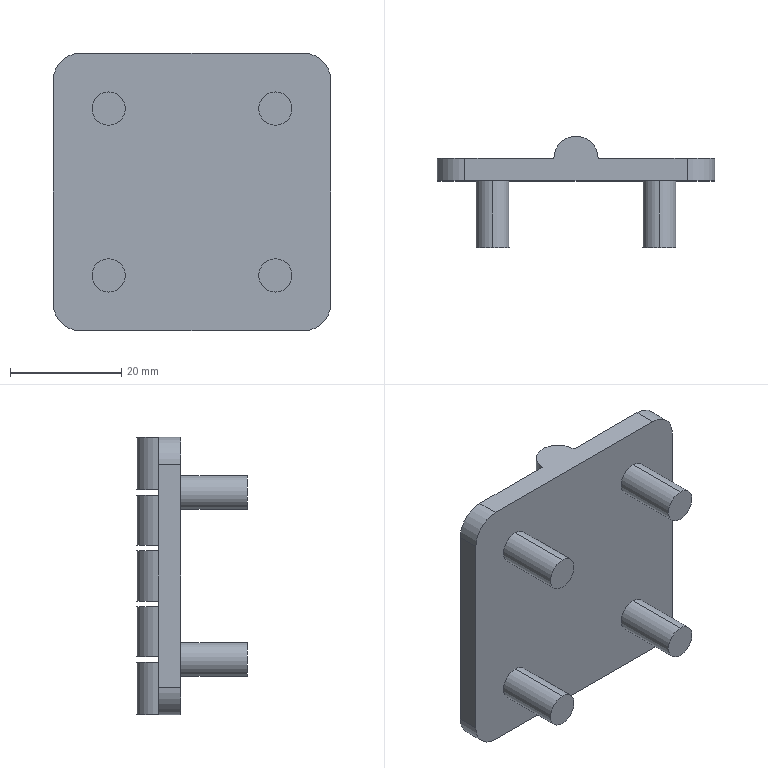Part | NX | features solid 2 | 1 solid | 35 faces | box 50 x 20 x 50 mm | volume 12427 mm3 | plane 18 | cylinder 17 | commonest cylinder face diameters 6 x8 8 x5 10 x4
STEP:
#1=CARTESIAN_POINT('',(675.,534.,662.));
#2=VERTEX_POINT('',#1);
#3=CARTESIAN_POINT('',(667.,534.,662.));
#4=VERTEX_POINT('',#3);
#5=CARTESIAN_POINT('',(671.,534.,662.));
#6=DIRECTION('',(0.,0.,1.));
#7=DIRECTION('',(0.,1.,0.));
#8=AXIS2_PLACEMENT_3D('',#5,#6,#7);
#9=CIRCLE('',#8,4.);
#10=EDGE_CURVE('',#2,#4,#9,.T.);
#11=ORIENTED_EDGE('',*,*,#10,.T.);
#12=CARTESIAN_POINT('',(676.528,534.,662.));
#13=DIRECTION('',(-1.,0.,0.));
#14=VECTOR('',#13,1000.);
#15=LINE('',#12,#14);
#16=EDGE_CURVE('',#2,#4,#15,.T.);
#17=ORIENTED_EDGE('',*,*,#16,.F.);
#18=EDGE_LOOP('',(#11,#17));
#19=FACE_BOUND('',#18,.T.);
#20=CARTESIAN_POINT('',(676.528,607.485,662.));
#21=DIRECTION('',(0.,0.,1.));
#22=DIRECTION('',(1.,0.,0.));
#23=AXIS2_PLACEMENT_3D('',#20,#21,#22);
#24=PLANE('',#23);
#25=ADVANCED_FACE('',(#19),#24,.T.);
#26=CARTESIAN_POINT('',(667.,534.,663.));
#27=VERTEX_POINT('',#26);
#28=CARTESIAN_POINT('',(675.,534.,663.));
#29=VERTEX_POINT('',#28);
#30=CARTESIAN_POINT('',(671.,534.,663.));
#31=DIRECTION('',(0.,0.,-1.));
#32=DIRECTION('',(0.,-1.,0.));
#33=AXIS2_PLACEMENT_3D('',#30,#31,#32);
#34=CIRCLE('',#33,4.);
#35=EDGE_CURVE('',#27,#29,#34,.T.);
#36=ORIENTED_EDGE('',*,*,#35,.T.);
#37=CARTESIAN_POINT('',(676.528,534.,663.));
#38=DIRECTION('',(1.,0.,0.));
#39=VECTOR('',#38,1000.);
#40=LINE('',#37,#39);
#41=EDGE_CURVE('',#27,#29,#40,.T.);
#42=ORIENTED_EDGE('',*,*,#41,.F.);
#43=EDGE_LOOP('',(#36,#42));
#44=FACE_BOUND('',#43,.T.);
#45=CARTESIAN_POINT('',(676.528,607.485,663.));
#46=DIRECTION('',(0.,0.,-1.));
#47=DIRECTION('',(0.,-1.,0.));
#48=AXIS2_PLACEMENT_3D('',#45,#46,#47);
#49=PLANE('',#48);
#50=ADVANCED_FACE('',(#44),#49,.T.);
#51=CARTESIAN_POINT('',(675.,534.,632.));
#52=VERTEX_POINT('',#51);
#53=CARTESIAN_POINT('',(667.,534.,632.));
#54=VERTEX_POINT('',#53);
#55=CARTESIAN_POINT('',(671.,534.,632.));
#56=DIRECTION('',(0.,0.,1.));
#57=DIRECTION('',(0.,1.,0.));
#58=AXIS2_PLACEMENT_3D('',#55,#56,#57);
#59=CIRCLE('',#58,4.);
#60=EDGE_CURVE('',#52,#54,#59,.T.);
#61=ORIENTED_EDGE('',*,*,#60,.T.);
#62=CARTESIAN_POINT('',(676.528,534.,632.));
#63=DIRECTION('',(-1.,0.,0.));
#64=VECTOR('',#63,1000.);
#65=LINE('',#62,#64);
#66=EDGE_CURVE('',#52,#54,#65,.T.);
#67=ORIENTED_EDGE('',*,*,#66,.F.);
#68=EDGE_LOOP('',(#61,#67));
#69=FACE_BOUND('',#68,.T.);
#70=CARTESIAN_POINT('',(676.528,607.485,632.));
#71=DIRECTION('',(0.,0.,1.));
#72=DIRECTION('',(1.,0.,0.));
#73=AXIS2_PLACEMENT_3D('',#70,#71,#72);
#74=PLANE('',#73);
#75=ADVANCED_FACE('',(#69),#74,.T.);
#76=CARTESIAN_POINT('',(667.,534.,633.));
#77=VERTEX_POINT('',#76);
#78=CARTESIAN_POINT('',(675.,534.,633.));
#79=VERTEX_POINT('',#78);
#80=CARTESIAN_POINT('',(671.,534.,633.));
#81=DIRECTION('',(0.,0.,-1.));
#82=DIRECTION('',(0.,-1.,0.));
#83=AXIS2_PLACEMENT_3D('',#80,#81,#82);
#84=CIRCLE('',#83,4.);
#85=EDGE_CURVE('',#77,#79,#84,.T.);
#86=ORIENTED_EDGE('',*,*,#85,.T.);
#87=CARTESIAN_POINT('',(676.528,534.,633.));
#88=DIRECTION('',(1.,0.,0.));
#89=VECTOR('',#88,1000.);
#90=LINE('',#87,#89);
#91=EDGE_CURVE('',#77,#79,#90,.T.);
#92=ORIENTED_EDGE('',*,*,#91,.F.);
#93=EDGE_LOOP('',(#86,#92));
#94=FACE_BOUND('',#93,.T.);
#95=CARTESIAN_POINT('',(676.528,607.485,633.));
#96=DIRECTION('',(0.,0.,-1.));
#97=DIRECTION('',(0.,-1.,0.));
#98=AXIS2_PLACEMENT_3D('',#95,#96,#97);
#99=PLANE('',#98);
#100=ADVANCED_FACE('',(#94),#99,.T.);
#101=CARTESIAN_POINT('',(675.,534.,642.));
#102=VERTEX_POINT('',#101);
#103=CARTESIAN_POINT('',(667.,534.,642.));
#104=VERTEX_POINT('',#103);
#105=CARTESIAN_POINT('',(671.,534.,642.));
#106=DIRECTION('',(0.,0.,1.));
#107=DIRECTION('',(0.,1.,0.));
#108=AXIS2_PLACEMENT_3D('',#105,#106,#107);
#109=CIRCLE('',#108,4.);
#110=EDGE_CURVE('',#102,#104,#109,.T.);
#111=ORIENTED_EDGE('',*,*,#110,.T.);
#112=CARTESIAN_POINT('',(676.528,534.,642.));
#113=DIRECTION('',(-1.,0.,0.));
#114=VECTOR('',#113,1000.);
#115=LINE('',#112,#114);
#116=EDGE_CURVE('',#102,#104,#115,.T.);
#117=ORIENTED_EDGE('',*,*,#116,.F.);
#118=EDGE_LOOP('',(#111,#117));
#119=FACE_BOUND('',#118,.T.);
#120=CARTESIAN_POINT('',(676.528,607.485,642.));
#121=DIRECTION('',(0.,0.,1.));
#122=DIRECTION('',(1.,0.,0.));
#123=AXIS2_PLACEMENT_3D('',#120,#121,#122);
#124=PLANE('',#123);
#125=ADVANCED_FACE('',(#119),#124,.T.);
#126=CARTESIAN_POINT('',(667.,534.,643.));
#127=VERTEX_POINT('',#126);
#128=CARTESIAN_POINT('',(675.,534.,643.));
#129=VERTEX_POINT('',#128);
#130=CARTESIAN_POINT('',(671.,534.,643.));
#131=DIRECTION('',(0.,0.,-1.));
#132=DIRECTION('',(0.,-1.,0.));
#133=AXIS2_PLACEMENT_3D('',#130,#131,#132);
#134=CIRCLE('',#133,4.);
#135=EDGE_CURVE('',#127,#129,#134,.T.);
#136=ORIENTED_EDGE('',*,*,#135,.T.);
#137=CARTESIAN_POINT('',(676.528,534.,643.));
#138=DIRECTION('',(1.,0.,0.));
#139=VECTOR('',#138,1000.);
#140=LINE('',#137,#139);
#141=EDGE_CURVE('',#127,#129,#140,.T.);
#142=ORIENTED_EDGE('',*,*,#141,.F.);
#143=EDGE_LOOP('',(#136,#142));
#144=FACE_BOUND('',#143,.T.);
#145=CARTESIAN_POINT('',(676.528,607.485,643.));
#146=DIRECTION('',(0.,0.,-1.));
#147=DIRECTION('',(0.,-1.,0.));
#148=AXIS2_PLACEMENT_3D('',#145,#146,#147);
#149=PLANE('',#148);
#150=ADVANCED_FACE('',(#144),#149,.T.);
#151=CARTESIAN_POINT('',(675.,534.,652.));
#152=VERTEX_POINT('',#151);
#153=CARTESIAN_POINT('',(667.,534.,652.));
#154=VERTEX_POINT('',#153);
#155=CARTESIAN_POINT('',(671.,534.,652.));
#156=DIRECTION('',(0.,0.,1.));
#157=DIRECTION('',(0.,1.,0.));
#158=AXIS2_PLACEMENT_3D('',#155,#156,#157);
#159=CIRCLE('',#158,4.);
#160=EDGE_CURVE('',#152,#154,#159,.T.);
#161=ORIENTED_EDGE('',*,*,#160,.T.);
#162=CARTESIAN_POINT('',(676.528,534.,652.));
#163=DIRECTION('',(-1.,0.,0.));
#164=VECTOR('',#163,1000.);
#165=LINE('',#162,#164);
#166=EDGE_CURVE('',#152,#154,#165,.T.);
#167=ORIENTED_EDGE('',*,*,#166,.F.);
#168=EDGE_LOOP('',(#161,#167));
#169=FACE_BOUND('',#168,.T.);
#170=CARTESIAN_POINT('',(676.528,607.485,652.));
#171=DIRECTION('',(0.,0.,1.));
#172=DIRECTION('',(1.,0.,0.));
#173=AXIS2_PLACEMENT_3D('',#170,#171,#172);
#174=PLANE('',#173);
#175=ADVANCED_FACE('',(#169),#174,.T.);
#176=CARTESIAN_POINT('',(667.,534.,653.));
#177=VERTEX_POINT('',#176);
#178=CARTESIAN_POINT('',(675.,534.,653.));
#179=VERTEX_POINT('',#178);
#180=CARTESIAN_POINT('',(671.,534.,653.));
#181=DIRECTION('',(0.,0.,-1.));
#182=DIRECTION('',(0.,-1.,0.));
#183=AXIS2_PLACEMENT_3D('',#180,#181,#182);
#184=CIRCLE('',#183,4.);
#185=EDGE_CURVE('',#177,#179,#184,.T.);
#186=ORIENTED_EDGE('',*,*,#185,.T.);
#187=CARTESIAN_POINT('',(676.528,534.,653.));
#188=DIRECTION('',(1.,0.,0.));
#189=VECTOR('',#188,1000.);
#190=LINE('',#187,#189);
#191=EDGE_CURVE('',#177,#179,#190,.T.);
#192=ORIENTED_EDGE('',*,*,#191,.F.);
#193=EDGE_LOOP('',(#186,#192));
#194=FACE_BOUND('',#193,.T.);
#195=CARTESIAN_POINT('',(676.528,607.485,653.));
#196=DIRECTION('',(0.,0.,-1.));
#197=DIRECTION('',(0.,-1.,0.));
#198=AXIS2_PLACEMENT_3D('',#195,#196,#197);
#199=PLANE('',#198);
#200=ADVANCED_FACE('',(#194),#199,.T.);
#201=CARTESIAN_POINT('',(686.,518.,629.5));
#202=VERTEX_POINT('',#201);
#203=CARTESIAN_POINT('',(686.,518.,635.5));
#204=VERTEX_POINT('',#203);
#205=CARTESIAN_POINT('',(686.,518.,632.5));
#206=DIRECTION('',(0.,1.,0.));
#207=DIRECTION('',(-1.,0.,0.));
#208=AXIS2_PLACEMENT_3D('',#205,#206,#207);
#209=CIRCLE('',#208,3.);
#210=EDGE_CURVE('',#202,#204,#209,.T.);
#211=ORIENTED_EDGE('',*,*,#210,.F.);
#212=CARTESIAN_POINT('',(686.,518.,632.5));
#213=DIRECTION('',(0.,1.,0.));
#214=DIRECTION('',(-1.,0.,0.));
#215=AXIS2_PLACEMENT_3D('',#212,#213,#214);
#216=CIRCLE('',#215,3.);
#217=EDGE_CURVE('',#204,#202,#216,.T.);
#218=ORIENTED_EDGE('',*,*,#217,.F.);
#219=EDGE_LOOP('',(#211,#218));
#220=FACE_BOUND('',#219,.T.);
#221=CARTESIAN_POINT('',(686.,518.,632.5));
#222=DIRECTION('',(0.,1.,0.));
#223=DIRECTION('',(1.,0.,0.));
#224=AXIS2_PLACEMENT_3D('',#221,#222,#223);
#225=PLANE('',#224);
#226=ADVANCED_FACE('',(#220),#225,.F.);
#227=CARTESIAN_POINT('',(686.,530.,635.5));
#228=VERTEX_POINT('',#227);
#229=CARTESIAN_POINT('',(686.,518.,635.5));
#230=DIRECTION('',(0.,1.,0.));
#231=VECTOR('',#230,1000.);
#232=LINE('',#229,#231);
#233=EDGE_CURVE('',#228,#204,#232,.F.);
#234=ORIENTED_EDGE('',*,*,#233,.T.);
#235=ORIENTED_EDGE('',*,*,#217,.T.);
#236=CARTESIAN_POINT('',(686.,530.,629.5));
#237=VERTEX_POINT('',#236);
#238=CARTESIAN_POINT('',(686.,518.,629.5));
#239=DIRECTION('',(0.,1.,0.));
#240=VECTOR('',#239,1000.);
#241=LINE('',#238,#240);
#242=EDGE_CURVE('',#202,#237,#241,.T.);
#243=ORIENTED_EDGE('',*,*,#242,.T.);
#244=CARTESIAN_POINT('',(686.,530.,632.5));
#245=DIRECTION('',(0.,-1.,0.));
#246=DIRECTION('',(0.,0.,1.));
#247=AXIS2_PLACEMENT_3D('',#244,#245,#246);
#248=CIRCLE('',#247,3.);
#249=EDGE_CURVE('',#237,#228,#248,.T.);
#250=ORIENTED_EDGE('',*,*,#249,.T.);
#251=EDGE_LOOP('',(#234,#235,#243,#250));
#252=FACE_BOUND('',#251,.T.);
#253=CARTESIAN_POINT('',(686.,518.,632.5));
#254=DIRECTION('',(0.,1.,0.));
#255=DIRECTION('',(0.,0.,-1.));
#256=AXIS2_PLACEMENT_3D('',#253,#254,#255);
#257=CYLINDRICAL_SURFACE('',#256,3.);
#258=ADVANCED_FACE('',(#252),#257,.T.);
#259=CARTESIAN_POINT('',(686.,518.,659.5));
#260=VERTEX_POINT('',#259);
#261=CARTESIAN_POINT('',(686.,518.,665.5));
#262=VERTEX_POINT('',#261);
#263=CARTESIAN_POINT('',(686.,518.,662.5));
#264=DIRECTION('',(0.,1.,0.));
#265=DIRECTION('',(-1.,0.,0.));
#266=AXIS2_PLACEMENT_3D('',#263,#264,#265);
#267=CIRCLE('',#266,3.);
#268=EDGE_CURVE('',#260,#262,#267,.T.);
#269=ORIENTED_EDGE('',*,*,#268,.F.);
#270=CARTESIAN_POINT('',(686.,518.,662.5));
#271=DIRECTION('',(0.,1.,0.));
#272=DIRECTION('',(-1.,0.,0.));
#273=AXIS2_PLACEMENT_3D('',#270,#271,#272);
#274=CIRCLE('',#273,3.);
#275=EDGE_CURVE('',#262,#260,#274,.T.);
#276=ORIENTED_EDGE('',*,*,#275,.F.);
#277=EDGE_LOOP('',(#269,#276));
#278=FACE_BOUND('',#277,.T.);
#279=CARTESIAN_POINT('',(686.,518.,662.5));
#280=DIRECTION('',(0.,1.,0.));
#281=DIRECTION('',(1.,0.,0.));
#282=AXIS2_PLACEMENT_3D('',#279,#280,#281);
#283=PLANE('',#282);
#284=ADVANCED_FACE('',(#278),#283,.F.);
#285=CARTESIAN_POINT('',(686.,530.,665.5));
#286=VERTEX_POINT('',#285);
#287=CARTESIAN_POINT('',(686.,518.,665.5));
#288=DIRECTION('',(0.,1.,0.));
#289=VECTOR('',#288,1000.);
#290=LINE('',#287,#289);
#291=EDGE_CURVE('',#286,#262,#290,.F.);
#292=ORIENTED_EDGE('',*,*,#291,.T.);
#293=ORIENTED_EDGE('',*,*,#275,.T.);
#294=CARTESIAN_POINT('',(686.,530.,659.5));
#295=VERTEX_POINT('',#294);
#296=CARTESIAN_POINT('',(686.,518.,659.5));
#297=DIRECTION('',(0.,1.,0.));
#298=VECTOR('',#297,1000.);
#299=LINE('',#296,#298);
#300=EDGE_CURVE('',#260,#295,#299,.T.);
#301=ORIENTED_EDGE('',*,*,#300,.T.);
#302=CARTESIAN_POINT('',(686.,530.,662.5));
#303=DIRECTION('',(0.,-1.,0.));
#304=DIRECTION('',(0.,0.,1.));
#305=AXIS2_PLACEMENT_3D('',#302,#303,#304);
#306=CIRCLE('',#305,3.);
#307=EDGE_CURVE('',#295,#286,#306,.T.);
#308=ORIENTED_EDGE('',*,*,#307,.T.);
#309=EDGE_LOOP('',(#292,#293,#301,#308));
#310=FACE_BOUND('',#309,.T.);
#311=CARTESIAN_POINT('',(686.,518.,662.5));
#312=DIRECTION('',(0.,1.,0.));
#313=DIRECTION('',(0.,0.,-1.));
#314=AXIS2_PLACEMENT_3D('',#311,#312,#313);
#315=CYLINDRICAL_SURFACE('',#314,3.);
#316=ADVANCED_FACE('',(#310),#315,.T.);
#317=CARTESIAN_POINT('',(656.,518.,659.5));
#318=VERTEX_POINT('',#317);
#319=CARTESIAN_POINT('',(656.,518.,665.5));
#320=VERTEX_POINT('',#319);
#321=CARTESIAN_POINT('',(656.,518.,662.5));
#322=DIRECTION('',(0.,1.,0.));
#323=DIRECTION('',(-1.,0.,0.));
#324=AXIS2_PLACEMENT_3D('',#321,#322,#323);
#325=CIRCLE('',#324,3.);
#326=EDGE_CURVE('',#318,#320,#325,.T.);
#327=ORIENTED_EDGE('',*,*,#326,.F.);
#328=CARTESIAN_POINT('',(656.,518.,662.5));
#329=DIRECTION('',(0.,1.,0.));
#330=DIRECTION('',(-1.,0.,0.));
#331=AXIS2_PLACEMENT_3D('',#328,#329,#330);
#332=CIRCLE('',#331,3.);
#333=EDGE_CURVE('',#320,#318,#332,.T.);
#334=ORIENTED_EDGE('',*,*,#333,.F.);
#335=EDGE_LOOP('',(#327,#334));
#336=FACE_BOUND('',#335,.T.);
#337=CARTESIAN_POINT('',(656.,518.,662.5));
#338=DIRECTION('',(0.,1.,0.));
#339=DIRECTION('',(1.,0.,0.));
#340=AXIS2_PLACEMENT_3D('',#337,#338,#339);
#341=PLANE('',#340);
#342=ADVANCED_FACE('',(#336),#341,.F.);
#343=CARTESIAN_POINT('',(656.,530.,665.5));
#344=VERTEX_POINT('',#343);
#345=CARTESIAN_POINT('',(656.,518.,665.5));
#346=DIRECTION('',(0.,1.,0.));
#347=VECTOR('',#346,1000.);
#348=LINE('',#345,#347);
#349=EDGE_CURVE('',#344,#320,#348,.F.);
#350=ORIENTED_EDGE('',*,*,#349,.T.);
#351=ORIENTED_EDGE('',*,*,#333,.T.);
#352=CARTESIAN_POINT('',(656.,530.,659.5));
#353=VERTEX_POINT('',#352);
#354=CARTESIAN_POINT('',(656.,518.,659.5));
#355=DIRECTION('',(0.,1.,0.));
#356=VECTOR('',#355,1000.);
#357=LINE('',#354,#356);
#358=EDGE_CURVE('',#318,#353,#357,.T.);
#359=ORIENTED_EDGE('',*,*,#358,.T.);
#360=CARTESIAN_POINT('',(656.,530.,662.5));
#361=DIRECTION('',(0.,-1.,0.));
#362=DIRECTION('',(0.,0.,1.));
#363=AXIS2_PLACEMENT_3D('',#360,#361,#362);
#364=CIRCLE('',#363,3.);
#365=EDGE_CURVE('',#353,#344,#364,.T.);
#366=ORIENTED_EDGE('',*,*,#365,.T.);
#367=EDGE_LOOP('',(#350,#351,#359,#366));
#368=FACE_BOUND('',#367,.T.);
#369=CARTESIAN_POINT('',(656.,518.,662.5));
#370=DIRECTION('',(0.,1.,0.));
#371=DIRECTION('',(0.,0.,-1.));
#372=AXIS2_PLACEMENT_3D('',#369,#370,#371);
#373=CYLINDRICAL_SURFACE('',#372,3.);
#374=ADVANCED_FACE('',(#368),#373,.T.);
#375=CARTESIAN_POINT('',(656.,518.,629.5));
#376=VERTEX_POINT('',#375);
#377=CARTESIAN_POINT('',(656.,518.,635.5));
#378=VERTEX_POINT('',#377);
#379=CARTESIAN_POINT('',(656.,518.,632.5));
#380=DIRECTION('',(0.,1.,0.));
#381=DIRECTION('',(-1.,0.,0.));
#382=AXIS2_PLACEMENT_3D('',#379,#380,#381);
#383=CIRCLE('',#382,3.);
#384=EDGE_CURVE('',#376,#378,#383,.T.);
#385=ORIENTED_EDGE('',*,*,#384,.F.);
#386=CARTESIAN_POINT('',(656.,518.,632.5));
#387=DIRECTION('',(0.,1.,0.));
#388=DIRECTION('',(-1.,0.,0.));
#389=AXIS2_PLACEMENT_3D('',#386,#387,#388);
#390=CIRCLE('',#389,3.);
#391=EDGE_CURVE('',#378,#376,#390,.T.);
#392=ORIENTED_EDGE('',*,*,#391,.F.);
#393=EDGE_LOOP('',(#385,#392));
#394=FACE_BOUND('',#393,.T.);
#395=CARTESIAN_POINT('',(656.,518.,632.5));
#396=DIRECTION('',(0.,1.,0.));
#397=DIRECTION('',(1.,0.,0.));
#398=AXIS2_PLACEMENT_3D('',#395,#396,#397);
#399=PLANE('',#398);
#400=ADVANCED_FACE('',(#394),#399,.F.);
#401=CARTESIAN_POINT('',(656.,530.,635.5));
#402=VERTEX_POINT('',#401);
#403=CARTESIAN_POINT('',(656.,518.,635.5));
#404=DIRECTION('',(0.,1.,0.));
#405=VECTOR('',#404,1000.);
#406=LINE('',#403,#405);
#407=EDGE_CURVE('',#378,#402,#406,.T.);
#408=ORIENTED_EDGE('',*,*,#407,.F.);
#409=ORIENTED_EDGE('',*,*,#391,.T.);
#410=CARTESIAN_POINT('',(656.,530.,629.5));
#411=VERTEX_POINT('',#410);
#412=CARTESIAN_POINT('',(656.,518.,629.5));
#413=DIRECTION('',(0.,1.,0.));
#414=VECTOR('',#413,1000.);
#415=LINE('',#412,#414);
#416=EDGE_CURVE('',#411,#376,#415,.F.);
#417=ORIENTED_EDGE('',*,*,#416,.F.);
#418=CARTESIAN_POINT('',(656.,530.,632.5));
#419=DIRECTION('',(0.,-1.,0.));
#420=DIRECTION('',(0.,0.,1.));
#421=AXIS2_PLACEMENT_3D('',#418,#419,#420);
#422=CIRCLE('',#421,3.);
#423=EDGE_CURVE('',#411,#402,#422,.T.);
#424=ORIENTED_EDGE('',*,*,#423,.T.);
#425=EDGE_LOOP('',(#408,#409,#417,#424));
#426=FACE_BOUND('',#425,.T.);
#427=CARTESIAN_POINT('',(656.,518.,632.5));
#428=DIRECTION('',(0.,1.,0.));
#429=DIRECTION('',(0.,0.,-1.));
#430=AXIS2_PLACEMENT_3D('',#427,#428,#429);
#431=CYLINDRICAL_SURFACE('',#430,3.);
#432=ADVANCED_FACE('',(#426),#431,.T.);
#433=CARTESIAN_POINT('',(646.,530.,627.5));
#434=VERTEX_POINT('',#433);
#435=CARTESIAN_POINT('',(651.,530.,622.5));
#436=VERTEX_POINT('',#435);
#437=CARTESIAN_POINT('',(651.,530.,627.5));
#438=DIRECTION('',(0.,-1.,0.));
#439=DIRECTION('',(0.,0.,1.));
#440=AXIS2_PLACEMENT_3D('',#437,#438,#439);
#441=CIRCLE('',#440,5.);
#442=EDGE_CURVE('',#434,#436,#441,.T.);
#443=ORIENTED_EDGE('',*,*,#442,.F.);
#444=CARTESIAN_POINT('',(646.,534.,627.5));
#445=VERTEX_POINT('',#444);
#446=CARTESIAN_POINT('',(646.,530.,627.5));
#447=DIRECTION('',(0.,-1.,0.));
#448=VECTOR('',#447,1000.);
#449=LINE('',#446,#448);
#450=EDGE_CURVE('',#445,#434,#449,.T.);
#451=ORIENTED_EDGE('',*,*,#450,.F.);
#452=CARTESIAN_POINT('',(651.,534.,622.5));
#453=VERTEX_POINT('',#452);
#454=CARTESIAN_POINT('',(651.,534.,627.5));
#455=DIRECTION('',(0.,1.,0.));
#456=DIRECTION('',(0.,0.,-1.));
#457=AXIS2_PLACEMENT_3D('',#454,#455,#456);
#458=CIRCLE('',#457,5.);
#459=EDGE_CURVE('',#453,#445,#458,.T.);
#460=ORIENTED_EDGE('',*,*,#459,.F.);
#461=CARTESIAN_POINT('',(651.,534.,622.5));
#462=DIRECTION('',(0.,1.,0.));
#463=VECTOR('',#462,1000.);
#464=LINE('',#461,#463);
#465=EDGE_CURVE('',#436,#453,#464,.T.);
#466=ORIENTED_EDGE('',*,*,#465,.F.);
#467=EDGE_LOOP('',(#443,#451,#460,#466));
#468=FACE_BOUND('',#467,.T.);
#469=CARTESIAN_POINT('',(651.,534.,627.5));
#470=DIRECTION('',(0.,-1.,0.));
#471=DIRECTION('',(0.,0.,1.));
#472=AXIS2_PLACEMENT_3D('',#469,#470,#471);
#473=CYLINDRICAL_SURFACE('',#472,5.);
#474=ADVANCED_FACE('',(#468),#473,.T.);
#475=CARTESIAN_POINT('',(691.,534.,672.5));
#476=VERTEX_POINT('',#475);
#477=CARTESIAN_POINT('',(696.,534.,667.5));
#478=VERTEX_POINT('',#477);
#479=CARTESIAN_POINT('',(691.,534.,667.5));
#480=DIRECTION('',(0.,1.,0.));
#481=DIRECTION('',(0.,0.,-1.));
#482=AXIS2_PLACEMENT_3D('',#479,#480,#481);
#483=CIRCLE('',#482,5.);
#484=EDGE_CURVE('',#476,#478,#483,.T.);
#485=ORIENTED_EDGE('',*,*,#484,.F.);
#486=CARTESIAN_POINT('',(691.,530.,672.5));
#487=VERTEX_POINT('',#486);
#488=CARTESIAN_POINT('',(691.,534.,672.5));
#489=DIRECTION('',(0.,1.,0.));
#490=VECTOR('',#489,1000.);
#491=LINE('',#488,#490);
#492=EDGE_CURVE('',#487,#476,#491,.T.);
#493=ORIENTED_EDGE('',*,*,#492,.F.);
#494=CARTESIAN_POINT('',(696.,530.,667.5));
#495=VERTEX_POINT('',#494);
#496=CARTESIAN_POINT('',(691.,530.,667.5));
#497=DIRECTION('',(0.,-1.,0.));
#498=DIRECTION('',(0.,0.,1.));
#499=AXIS2_PLACEMENT_3D('',#496,#497,#498);
#500=CIRCLE('',#499,5.);
#501=EDGE_CURVE('',#495,#487,#500,.T.);
#502=ORIENTED_EDGE('',*,*,#501,.F.);
#503=CARTESIAN_POINT('',(696.,534.,667.5));
#504=DIRECTION('',(0.,-1.,0.));
#505=VECTOR('',#504,1000.);
#506=LINE('',#503,#505);
#507=EDGE_CURVE('',#478,#495,#506,.T.);
#508=ORIENTED_EDGE('',*,*,#507,.F.);
#509=EDGE_LOOP('',(#485,#493,#502,#508));
#510=FACE_BOUND('',#509,.T.);
#511=CARTESIAN_POINT('',(691.,534.,667.5));
#512=DIRECTION('',(0.,-1.,0.));
#513=DIRECTION('',(0.,0.,1.));
#514=AXIS2_PLACEMENT_3D('',#511,#512,#513);
#515=CYLINDRICAL_SURFACE('',#514,5.);
#516=ADVANCED_FACE('',(#510),#515,.T.);
#517=CARTESIAN_POINT('',(696.,534.,627.5));
#518=VERTEX_POINT('',#517);
#519=CARTESIAN_POINT('',(691.,534.,622.5));
#520=VERTEX_POINT('',#519);
#521=CARTESIAN_POINT('',(691.,534.,627.5));
#522=DIRECTION('',(0.,1.,0.));
#523=DIRECTION('',(0.,0.,-1.));
#524=AXIS2_PLACEMENT_3D('',#521,#522,#523);
#525=CIRCLE('',#524,5.);
#526=EDGE_CURVE('',#518,#520,#525,.T.);
#527=ORIENTED_EDGE('',*,*,#526,.F.);
#528=CARTESIAN_POINT('',(696.,530.,627.5));
#529=VERTEX_POINT('',#528);
#530=CARTESIAN_POINT('',(696.,534.,627.5));
#531=DIRECTION('',(0.,1.,0.));
#532=VECTOR('',#531,1000.);
#533=LINE('',#530,#532);
#534=EDGE_CURVE('',#529,#518,#533,.T.);
#535=ORIENTED_EDGE('',*,*,#534,.F.);
#536=CARTESIAN_POINT('',(691.,530.,622.5));
#537=VERTEX_POINT('',#536);
#538=CARTESIAN_POINT('',(691.,530.,627.5));
#539=DIRECTION('',(0.,-1.,0.));
#540=DIRECTION('',(0.,0.,1.));
#541=AXIS2_PLACEMENT_3D('',#538,#539,#540);
#542=CIRCLE('',#541,5.);
#543=EDGE_CURVE('',#537,#529,#542,.T.);
#544=ORIENTED_EDGE('',*,*,#543,.F.);
#545=CARTESIAN_POINT('',(691.,530.,622.5));
#546=DIRECTION('',(0.,-1.,0.));
#547=VECTOR('',#546,1000.);
#548=LINE('',#545,#547);
#549=EDGE_CURVE('',#520,#537,#548,.T.);
#550=ORIENTED_EDGE('',*,*,#549,.F.);
#551=EDGE_LOOP('',(#527,#535,#544,#550));
#552=FACE_BOUND('',#551,.T.);
#553=CARTESIAN_POINT('',(691.,534.,627.5));
#554=DIRECTION('',(0.,1.,0.));
#555=DIRECTION('',(0.,0.,-1.));
#556=AXIS2_PLACEMENT_3D('',#553,#554,#555);
#557=CYLINDRICAL_SURFACE('',#556,5.);
#558=ADVANCED_FACE('',(#552),#557,.T.);
#559=CARTESIAN_POINT('',(651.,530.,672.5));
#560=VERTEX_POINT('',#559);
#561=CARTESIAN_POINT('',(646.,530.,667.5));
#562=VERTEX_POINT('',#561);
#563=CARTESIAN_POINT('',(651.,530.,667.5));
#564=DIRECTION('',(0.,-1.,0.));
#565=DIRECTION('',(0.,0.,1.));
#566=AXIS2_PLACEMENT_3D('',#563,#564,#565);
#567=CIRCLE('',#566,5.);
#568=EDGE_CURVE('',#560,#562,#567,.T.);
#569=ORIENTED_EDGE('',*,*,#568,.F.);
#570=CARTESIAN_POINT('',(651.,534.,672.5));
#571=VERTEX_POINT('',#570);
#572=CARTESIAN_POINT('',(651.,534.,672.5));
#573=DIRECTION('',(0.,-1.,0.));
#574=VECTOR('',#573,1000.);
#575=LINE('',#572,#574);
#576=EDGE_CURVE('',#571,#560,#575,.T.);
#577=ORIENTED_EDGE('',*,*,#576,.F.);
#578=CARTESIAN_POINT('',(646.,534.,667.5));
#579=VERTEX_POINT('',#578);
#580=CARTESIAN_POINT('',(651.,534.,667.5));
#581=DIRECTION('',(0.,1.,0.));
#582=DIRECTION('',(0.,0.,-1.));
#583=AXIS2_PLACEMENT_3D('',#580,#581,#582);
#584=CIRCLE('',#583,5.);
#585=EDGE_CURVE('',#579,#571,#584,.T.);
#586=ORIENTED_EDGE('',*,*,#585,.F.);
#587=CARTESIAN_POINT('',(646.,530.,667.5));
#588=DIRECTION('',(0.,1.,0.));
#589=VECTOR('',#588,1000.);
#590=LINE('',#587,#589);
#591=EDGE_CURVE('',#562,#579,#590,.T.);
#592=ORIENTED_EDGE('',*,*,#591,.F.);
#593=EDGE_LOOP('',(#569,#577,#586,#592));
#594=FACE_BOUND('',#593,.T.);
#595=CARTESIAN_POINT('',(651.,530.,667.5));
#596=DIRECTION('',(0.,1.,0.));
#597=DIRECTION('',(0.,0.,-1.));
#598=AXIS2_PLACEMENT_3D('',#595,#596,#597);
#599=CYLINDRICAL_SURFACE('',#598,5.);
#600=ADVANCED_FACE('',(#594),#599,.T.);
#601=CARTESIAN_POINT('',(646.,534.,672.5));
#602=DIRECTION('',(0.,0.,-1.));
#603=VECTOR('',#602,1000.);
#604=LINE('',#601,#603);
#605=EDGE_CURVE('',#579,#445,#604,.T.);
#606=ORIENTED_EDGE('',*,*,#605,.T.);
#607=ORIENTED_EDGE('',*,*,#450,.T.);
#608=CARTESIAN_POINT('',(646.,530.,672.5));
#609=DIRECTION('',(0.,0.,-1.));
#610=VECTOR('',#609,1000.);
#611=LINE('',#608,#610);
#612=EDGE_CURVE('',#562,#434,#611,.T.);
#613=ORIENTED_EDGE('',*,*,#612,.F.);
#614=ORIENTED_EDGE('',*,*,#591,.T.);
#615=EDGE_LOOP('',(#606,#607,#613,#614));
#616=FACE_BOUND('',#615,.T.);
#617=CARTESIAN_POINT('',(646.,530.,672.5));
#618=DIRECTION('',(-1.,0.,0.));
#619=DIRECTION('',(0.,0.,1.));
#620=AXIS2_PLACEMENT_3D('',#617,#618,#619);
#621=PLANE('',#620);
#622=ADVANCED_FACE('',(#616),#621,.T.);
#623=CARTESIAN_POINT('',(696.,534.,672.5));
#624=DIRECTION('',(0.,0.,-1.));
#625=VECTOR('',#624,1000.);
#626=LINE('',#623,#625);
#627=EDGE_CURVE('',#478,#518,#626,.T.);
#628=ORIENTED_EDGE('',*,*,#627,.F.);
#629=ORIENTED_EDGE('',*,*,#507,.T.);
#630=CARTESIAN_POINT('',(696.,530.,672.5));
#631=DIRECTION('',(0.,0.,-1.));
#632=VECTOR('',#631,1000.);
#633=LINE('',#630,#632);
#634=EDGE_CURVE('',#495,#529,#633,.T.);
#635=ORIENTED_EDGE('',*,*,#634,.T.);
#636=ORIENTED_EDGE('',*,*,#534,.T.);
#637=EDGE_LOOP('',(#628,#629,#635,#636));
#638=FACE_BOUND('',#637,.T.);
#639=CARTESIAN_POINT('',(696.,534.,672.5));
#640=DIRECTION('',(1.,0.,0.));
#641=DIRECTION('',(0.,0.,1.));
#642=AXIS2_PLACEMENT_3D('',#639,#640,#641);
#643=PLANE('',#642);
#644=ADVANCED_FACE('',(#638),#643,.T.);
#645=ORIENTED_EDGE('',*,*,#141,.T.);
#646=CARTESIAN_POINT('',(675.,534.,672.5));
#647=DIRECTION('',(0.,0.,-1.));
#648=VECTOR('',#647,1000.);
#649=LINE('',#646,#648);
#650=EDGE_CURVE('',#152,#129,#649,.T.);
#651=ORIENTED_EDGE('',*,*,#650,.F.);
#652=ORIENTED_EDGE('',*,*,#166,.T.);
#653=CARTESIAN_POINT('',(667.,534.,672.5));
#654=DIRECTION('',(0.,0.,1.));
#655=VECTOR('',#654,1000.);
#656=LINE('',#653,#655);
#657=EDGE_CURVE('',#127,#154,#656,.T.);
#658=ORIENTED_EDGE('',*,*,#657,.F.);
#659=EDGE_LOOP('',(#645,#651,#652,#658));
#660=FACE_BOUND('',#659,.T.);
#661=ORIENTED_EDGE('',*,*,#91,.T.);
#662=CARTESIAN_POINT('',(675.,534.,672.5));
#663=DIRECTION('',(0.,0.,-1.));
#664=VECTOR('',#663,1000.);
#665=LINE('',#662,#664);
#666=EDGE_CURVE('',#102,#79,#665,.T.);
#667=ORIENTED_EDGE('',*,*,#666,.F.);
#668=ORIENTED_EDGE('',*,*,#116,.T.);
#669=CARTESIAN_POINT('',(667.,534.,672.5));
#670=DIRECTION('',(0.,0.,1.));
#671=VECTOR('',#670,1000.);
#672=LINE('',#669,#671);
#673=EDGE_CURVE('',#77,#104,#672,.T.);
#674=ORIENTED_EDGE('',*,*,#673,.F.);
#675=EDGE_LOOP('',(#661,#667,#668,#674));
#676=FACE_BOUND('',#675,.T.);
#677=ORIENTED_EDGE('',*,*,#16,.T.);
#678=CARTESIAN_POINT('',(667.,534.,672.5));
#679=DIRECTION('',(0.,0.,1.));
#680=VECTOR('',#679,1000.);
#681=LINE('',#678,#680);
#682=EDGE_CURVE('',#177,#4,#681,.T.);
#683=ORIENTED_EDGE('',*,*,#682,.F.);
#684=ORIENTED_EDGE('',*,*,#191,.T.);
#685=CARTESIAN_POINT('',(675.,534.,672.5));
#686=DIRECTION('',(0.,0.,-1.));
#687=VECTOR('',#686,1000.);
#688=LINE('',#685,#687);
#689=EDGE_CURVE('',#2,#179,#688,.T.);
#690=ORIENTED_EDGE('',*,*,#689,.F.);
#691=EDGE_LOOP('',(#677,#683,#684,#690));
#692=FACE_BOUND('',#691,.T.);
#693=ORIENTED_EDGE('',*,*,#41,.T.);
#694=CARTESIAN_POINT('',(675.,534.,672.5));
#695=VERTEX_POINT('',#694);
#696=CARTESIAN_POINT('',(675.,534.,672.5));
#697=DIRECTION('',(0.,0.,-1.));
#698=VECTOR('',#697,1000.);
#699=LINE('',#696,#698);
#700=EDGE_CURVE('',#695,#29,#699,.T.);
#701=ORIENTED_EDGE('',*,*,#700,.F.);
#702=CARTESIAN_POINT('',(646.,534.,672.5));
#703=DIRECTION('',(1.,0.,0.));
#704=VECTOR('',#703,1000.);
#705=LINE('',#702,#704);
#706=EDGE_CURVE('',#695,#476,#705,.T.);
#707=ORIENTED_EDGE('',*,*,#706,.T.);
#708=ORIENTED_EDGE('',*,*,#484,.T.);
#709=ORIENTED_EDGE('',*,*,#627,.T.);
#710=ORIENTED_EDGE('',*,*,#526,.T.);
#711=CARTESIAN_POINT('',(675.,534.,622.5));
#712=VERTEX_POINT('',#711);
#713=CARTESIAN_POINT('',(646.,534.,622.5));
#714=DIRECTION('',(1.,0.,0.));
#715=VECTOR('',#714,1000.);
#716=LINE('',#713,#715);
#717=EDGE_CURVE('',#712,#520,#716,.T.);
#718=ORIENTED_EDGE('',*,*,#717,.F.);
#719=CARTESIAN_POINT('',(675.,534.,672.5));
#720=DIRECTION('',(0.,0.,-1.));
#721=VECTOR('',#720,1000.);
#722=LINE('',#719,#721);
#723=EDGE_CURVE('',#52,#712,#722,.T.);
#724=ORIENTED_EDGE('',*,*,#723,.F.);
#725=ORIENTED_EDGE('',*,*,#66,.T.);
#726=CARTESIAN_POINT('',(667.,534.,622.5));
#727=VERTEX_POINT('',#726);
#728=CARTESIAN_POINT('',(667.,534.,672.5));
#729=DIRECTION('',(0.,0.,1.));
#730=VECTOR('',#729,1000.);
#731=LINE('',#728,#730);
#732=EDGE_CURVE('',#727,#54,#731,.T.);
#733=ORIENTED_EDGE('',*,*,#732,.F.);
#734=CARTESIAN_POINT('',(646.,534.,622.5));
#735=DIRECTION('',(1.,0.,0.));
#736=VECTOR('',#735,1000.);
#737=LINE('',#734,#736);
#738=EDGE_CURVE('',#453,#727,#737,.T.);
#739=ORIENTED_EDGE('',*,*,#738,.F.);
#740=ORIENTED_EDGE('',*,*,#459,.T.);
#741=ORIENTED_EDGE('',*,*,#605,.F.);
#742=ORIENTED_EDGE('',*,*,#585,.T.);
#743=CARTESIAN_POINT('',(667.,534.,672.5));
#744=VERTEX_POINT('',#743);
#745=CARTESIAN_POINT('',(646.,534.,672.5));
#746=DIRECTION('',(1.,0.,0.));
#747=VECTOR('',#746,1000.);
#748=LINE('',#745,#747);
#749=EDGE_CURVE('',#571,#744,#748,.T.);
#750=ORIENTED_EDGE('',*,*,#749,.T.);
#751=CARTESIAN_POINT('',(667.,534.,672.5));
#752=DIRECTION('',(0.,0.,1.));
#753=VECTOR('',#752,1000.);
#754=LINE('',#751,#753);
#755=EDGE_CURVE('',#27,#744,#754,.T.);
#756=ORIENTED_EDGE('',*,*,#755,.F.);
#757=EDGE_LOOP('',(#693,#701,#707,#708,#709,#710,#718,#724,#725,#733,#739,#740,#741,#742,#750,#756));
#758=FACE_BOUND('',#757,.T.);
#759=CARTESIAN_POINT('',(646.,534.,672.5));
#760=DIRECTION('',(0.,1.,0.));
#761=DIRECTION('',(1.,0.,0.));
#762=AXIS2_PLACEMENT_3D('',#759,#760,#761);
#763=PLANE('',#762);
#764=ADVANCED_FACE('',(#660,#676,#692,#758),#763,.T.);
#765=ORIENTED_EDGE('',*,*,#423,.F.);
#766=CARTESIAN_POINT('',(656.,530.,632.5));
#767=DIRECTION('',(0.,-1.,0.));
#768=DIRECTION('',(0.,0.,1.));
#769=AXIS2_PLACEMENT_3D('',#766,#767,#768);
#770=CIRCLE('',#769,3.);
#771=EDGE_CURVE('',#402,#411,#770,.T.);
#772=ORIENTED_EDGE('',*,*,#771,.F.);
#773=EDGE_LOOP('',(#765,#772));
#774=FACE_BOUND('',#773,.T.);
#775=ORIENTED_EDGE('',*,*,#365,.F.);
#776=CARTESIAN_POINT('',(656.,530.,662.5));
#777=DIRECTION('',(0.,-1.,0.));
#778=DIRECTION('',(0.,0.,1.));
#779=AXIS2_PLACEMENT_3D('',#776,#777,#778);
#780=CIRCLE('',#779,3.);
#781=EDGE_CURVE('',#344,#353,#780,.T.);
#782=ORIENTED_EDGE('',*,*,#781,.F.);
#783=EDGE_LOOP('',(#775,#782));
#784=FACE_BOUND('',#783,.T.);
#785=ORIENTED_EDGE('',*,*,#307,.F.);
#786=CARTESIAN_POINT('',(686.,530.,662.5));
#787=DIRECTION('',(0.,-1.,0.));
#788=DIRECTION('',(0.,0.,1.));
#789=AXIS2_PLACEMENT_3D('',#786,#787,#788);
#790=CIRCLE('',#789,3.);
#791=EDGE_CURVE('',#286,#295,#790,.T.);
#792=ORIENTED_EDGE('',*,*,#791,.F.);
#793=EDGE_LOOP('',(#785,#792));
#794=FACE_BOUND('',#793,.T.);
#795=ORIENTED_EDGE('',*,*,#249,.F.);
#796=CARTESIAN_POINT('',(686.,530.,632.5));
#797=DIRECTION('',(0.,-1.,0.));
#798=DIRECTION('',(0.,0.,1.));
#799=AXIS2_PLACEMENT_3D('',#796,#797,#798);
#800=CIRCLE('',#799,3.);
#801=EDGE_CURVE('',#228,#237,#800,.T.);
#802=ORIENTED_EDGE('',*,*,#801,.F.);
#803=EDGE_LOOP('',(#795,#802));
#804=FACE_BOUND('',#803,.T.);
#805=ORIENTED_EDGE('',*,*,#612,.T.);
#806=ORIENTED_EDGE('',*,*,#442,.T.);
#807=CARTESIAN_POINT('',(696.,530.,622.5));
#808=DIRECTION('',(-1.,0.,0.));
#809=VECTOR('',#808,1000.);
#810=LINE('',#807,#809);
#811=EDGE_CURVE('',#537,#436,#810,.T.);
#812=ORIENTED_EDGE('',*,*,#811,.F.);
#813=ORIENTED_EDGE('',*,*,#543,.T.);
#814=ORIENTED_EDGE('',*,*,#634,.F.);
#815=ORIENTED_EDGE('',*,*,#501,.T.);
#816=CARTESIAN_POINT('',(696.,530.,672.5));
#817=DIRECTION('',(-1.,0.,0.));
#818=VECTOR('',#817,1000.);
#819=LINE('',#816,#818);
#820=EDGE_CURVE('',#487,#560,#819,.T.);
#821=ORIENTED_EDGE('',*,*,#820,.T.);
#822=ORIENTED_EDGE('',*,*,#568,.T.);
#823=EDGE_LOOP('',(#805,#806,#812,#813,#814,#815,#821,#822));
#824=FACE_BOUND('',#823,.T.);
#825=CARTESIAN_POINT('',(696.,530.,672.5));
#826=DIRECTION('',(0.,-1.,0.));
#827=DIRECTION('',(-1.,0.,0.));
#828=AXIS2_PLACEMENT_3D('',#825,#826,#827);
#829=PLANE('',#828);
#830=ADVANCED_FACE('',(#774,#784,#794,#804,#824),#829,.T.);
#831=ORIENTED_EDGE('',*,*,#811,.T.);
#832=ORIENTED_EDGE('',*,*,#465,.T.);
#833=ORIENTED_EDGE('',*,*,#738,.T.);
#834=CARTESIAN_POINT('',(671.,534.,622.5));
#835=DIRECTION('',(0.,0.,1.));
#836=DIRECTION('',(-1.,0.,0.));
#837=AXIS2_PLACEMENT_3D('',#834,#835,#836);
#838=CIRCLE('',#837,4.);
#839=EDGE_CURVE('',#712,#727,#838,.T.);
#840=ORIENTED_EDGE('',*,*,#839,.F.);
#841=ORIENTED_EDGE('',*,*,#717,.T.);
#842=ORIENTED_EDGE('',*,*,#549,.T.);
#843=EDGE_LOOP('',(#831,#832,#833,#840,#841,#842));
#844=FACE_BOUND('',#843,.T.);
#845=CARTESIAN_POINT('',(671.,534.,622.5));
#846=DIRECTION('',(0.,0.,1.));
#847=DIRECTION('',(1.,0.,0.));
#848=AXIS2_PLACEMENT_3D('',#845,#846,#847);
#849=PLANE('',#848);
#850=ADVANCED_FACE('',(#844),#849,.F.);
#851=ORIENTED_EDGE('',*,*,#820,.F.);
#852=ORIENTED_EDGE('',*,*,#492,.T.);
#853=ORIENTED_EDGE('',*,*,#706,.F.);
#854=CARTESIAN_POINT('',(671.,534.,672.5));
#855=DIRECTION('',(0.,0.,1.));
#856=DIRECTION('',(-1.,0.,0.));
#857=AXIS2_PLACEMENT_3D('',#854,#855,#856);
#858=CIRCLE('',#857,4.);
#859=EDGE_CURVE('',#695,#744,#858,.T.);
#860=ORIENTED_EDGE('',*,*,#859,.T.);
#861=ORIENTED_EDGE('',*,*,#749,.F.);
#862=ORIENTED_EDGE('',*,*,#576,.T.);
#863=EDGE_LOOP('',(#851,#852,#853,#860,#861,#862));
#864=FACE_BOUND('',#863,.T.);
#865=CARTESIAN_POINT('',(671.,534.,672.5));
#866=DIRECTION('',(0.,0.,1.));
#867=DIRECTION('',(1.,0.,0.));
#868=AXIS2_PLACEMENT_3D('',#865,#866,#867);
#869=PLANE('',#868);
#870=ADVANCED_FACE('',(#864),#869,.T.);
#871=ORIENTED_EDGE('',*,*,#135,.F.);
#872=ORIENTED_EDGE('',*,*,#657,.T.);
#873=ORIENTED_EDGE('',*,*,#160,.F.);
#874=ORIENTED_EDGE('',*,*,#650,.T.);
#875=EDGE_LOOP('',(#871,#872,#873,#874));
#876=FACE_BOUND('',#875,.T.);
#877=CARTESIAN_POINT('',(671.,534.,672.5));
#878=DIRECTION('',(0.,0.,-1.));
#879=DIRECTION('',(0.,-1.,0.));
#880=AXIS2_PLACEMENT_3D('',#877,#878,#879);
#881=CYLINDRICAL_SURFACE('',#880,4.);
#882=ADVANCED_FACE('',(#876),#881,.T.);
#883=ORIENTED_EDGE('',*,*,#60,.F.);
#884=ORIENTED_EDGE('',*,*,#723,.T.);
#885=ORIENTED_EDGE('',*,*,#839,.T.);
#886=ORIENTED_EDGE('',*,*,#732,.T.);
#887=EDGE_LOOP('',(#883,#884,#885,#886));
#888=FACE_BOUND('',#887,.T.);
#889=CARTESIAN_POINT('',(671.,534.,672.5));
#890=DIRECTION('',(0.,0.,-1.));
#891=DIRECTION('',(0.,-1.,0.));
#892=AXIS2_PLACEMENT_3D('',#889,#890,#891);
#893=CYLINDRICAL_SURFACE('',#892,4.);
#894=ADVANCED_FACE('',(#888),#893,.T.);
#895=ORIENTED_EDGE('',*,*,#85,.F.);
#896=ORIENTED_EDGE('',*,*,#673,.T.);
#897=ORIENTED_EDGE('',*,*,#110,.F.);
#898=ORIENTED_EDGE('',*,*,#666,.T.);
#899=EDGE_LOOP('',(#895,#896,#897,#898));
#900=FACE_BOUND('',#899,.T.);
#901=CARTESIAN_POINT('',(671.,534.,672.5));
#902=DIRECTION('',(0.,0.,-1.));
#903=DIRECTION('',(0.,-1.,0.));
#904=AXIS2_PLACEMENT_3D('',#901,#902,#903);
#905=CYLINDRICAL_SURFACE('',#904,4.);
#906=ADVANCED_FACE('',(#900),#905,.T.);
#907=ORIENTED_EDGE('',*,*,#10,.F.);
#908=ORIENTED_EDGE('',*,*,#689,.T.);
#909=ORIENTED_EDGE('',*,*,#185,.F.);
#910=ORIENTED_EDGE('',*,*,#682,.T.);
#911=EDGE_LOOP('',(#907,#908,#909,#910));
#912=FACE_BOUND('',#911,.T.);
#913=CARTESIAN_POINT('',(671.,534.,672.5));
#914=DIRECTION('',(0.,0.,-1.));
#915=DIRECTION('',(0.,-1.,0.));
#916=AXIS2_PLACEMENT_3D('',#913,#914,#915);
#917=CYLINDRICAL_SURFACE('',#916,4.);
#918=ADVANCED_FACE('',(#912),#917,.T.);
#919=ORIENTED_EDGE('',*,*,#35,.F.);
#920=ORIENTED_EDGE('',*,*,#755,.T.);
#921=ORIENTED_EDGE('',*,*,#859,.F.);
#922=ORIENTED_EDGE('',*,*,#700,.T.);
#923=EDGE_LOOP('',(#919,#920,#921,#922));
#924=FACE_BOUND('',#923,.T.);
#925=CARTESIAN_POINT('',(671.,534.,672.5));
#926=DIRECTION('',(0.,0.,-1.));
#927=DIRECTION('',(0.,-1.,0.));
#928=AXIS2_PLACEMENT_3D('',#925,#926,#927);
#929=CYLINDRICAL_SURFACE('',#928,4.);
#930=ADVANCED_FACE('',(#924),#929,.T.);
#931=ORIENTED_EDGE('',*,*,#384,.T.);
#932=ORIENTED_EDGE('',*,*,#407,.T.);
#933=ORIENTED_EDGE('',*,*,#771,.T.);
#934=ORIENTED_EDGE('',*,*,#416,.T.);
#935=EDGE_LOOP('',(#931,#932,#933,#934));
#936=FACE_BOUND('',#935,.T.);
#937=CARTESIAN_POINT('',(656.,518.,632.5));
#938=DIRECTION('',(0.,1.,0.));
#939=DIRECTION('',(0.,0.,-1.));
#940=AXIS2_PLACEMENT_3D('',#937,#938,#939);
#941=CYLINDRICAL_SURFACE('',#940,3.);
#942=ADVANCED_FACE('',(#936),#941,.T.);
#943=ORIENTED_EDGE('',*,*,#326,.T.);
#944=ORIENTED_EDGE('',*,*,#349,.F.);
#945=ORIENTED_EDGE('',*,*,#781,.T.);
#946=ORIENTED_EDGE('',*,*,#358,.F.);
#947=EDGE_LOOP('',(#943,#944,#945,#946));
#948=FACE_BOUND('',#947,.T.);
#949=CARTESIAN_POINT('',(656.,518.,662.5));
#950=DIRECTION('',(0.,1.,0.));
#951=DIRECTION('',(0.,0.,-1.));
#952=AXIS2_PLACEMENT_3D('',#949,#950,#951);
#953=CYLINDRICAL_SURFACE('',#952,3.);
#954=ADVANCED_FACE('',(#948),#953,.T.);
#955=ORIENTED_EDGE('',*,*,#268,.T.);
#956=ORIENTED_EDGE('',*,*,#291,.F.);
#957=ORIENTED_EDGE('',*,*,#791,.T.);
#958=ORIENTED_EDGE('',*,*,#300,.F.);
#959=EDGE_LOOP('',(#955,#956,#957,#958));
#960=FACE_BOUND('',#959,.T.);
#961=CARTESIAN_POINT('',(686.,518.,662.5));
#962=DIRECTION('',(0.,1.,0.));
#963=DIRECTION('',(0.,0.,-1.));
#964=AXIS2_PLACEMENT_3D('',#961,#962,#963);
#965=CYLINDRICAL_SURFACE('',#964,3.);
#966=ADVANCED_FACE('',(#960),#965,.T.);
#967=ORIENTED_EDGE('',*,*,#210,.T.);
#968=ORIENTED_EDGE('',*,*,#233,.F.);
#969=ORIENTED_EDGE('',*,*,#801,.T.);
#970=ORIENTED_EDGE('',*,*,#242,.F.);
#971=EDGE_LOOP('',(#967,#968,#969,#970));
#972=FACE_BOUND('',#971,.T.);
#973=CARTESIAN_POINT('',(686.,518.,632.5));
#974=DIRECTION('',(0.,1.,0.));
#975=DIRECTION('',(0.,0.,-1.));
#976=AXIS2_PLACEMENT_3D('',#973,#974,#975);
#977=CYLINDRICAL_SURFACE('',#976,3.);
#978=ADVANCED_FACE('',(#972),#977,.T.);
#979=CLOSED_SHELL('',(#25,#50,#75,#100,#125,#150,#175,#200,#226,#258,#284,#316,#342,#374,#400,#432,#474,#516,#558,#600,#622,#644,#764,#830,#850,#870,#882,#894,#906,#918,#930,#942,#954,#966,#978));
#980=MANIFOLD_SOLID_BREP('',#979);
#981=(LENGTH_UNIT()NAMED_UNIT(*)SI_UNIT(.MILLI.,.METRE.));
#982=UNCERTAINTY_MEASURE_WITH_UNIT(LENGTH_MEASURE(0.00001),#981,'','');
#983=(NAMED_UNIT(*)PLANE_ANGLE_UNIT()SI_UNIT($,.RADIAN.));
#984=(NAMED_UNIT(*)SI_UNIT($,.STERADIAN.)SOLID_ANGLE_UNIT());
#985=(GEOMETRIC_REPRESENTATION_CONTEXT(3)GLOBAL_UNCERTAINTY_ASSIGNED_CONTEXT((#982))GLOBAL_UNIT_ASSIGNED_CONTEXT((#981,#983,#984))REPRESENTATION_CONTEXT('',''));
#986=ADVANCED_BREP_SHAPE_REPRESENTATION('',(#980),#985);